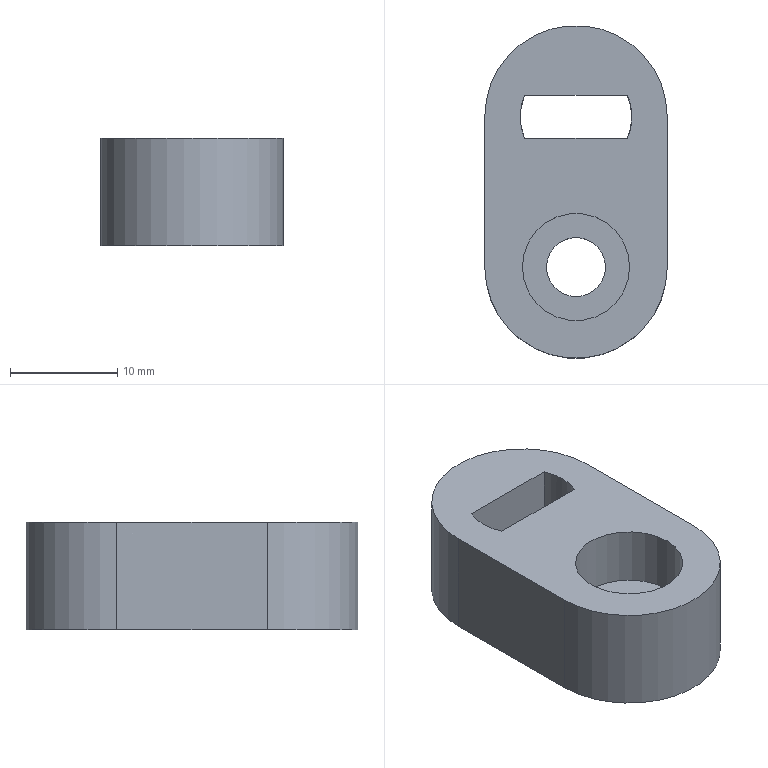Part | STEP file | lll_id290_x_t | 1 solid | 14 faces | box 17 x 31 x 10 mm | volume 3483 mm3 | plane 9 | cylinder 5 | commonest cylinder face diameters 17 x2 5.5 x1 10 x1 10.4 x1
STEP:
#1=CARTESIAN_POINT('',(5.,92.,-10.));
#2=VERTEX_POINT('',#1);
#3=CARTESIAN_POINT('',(0.,92.,-10.));
#4=DIRECTION('',(0.,0.,-1.));
#5=DIRECTION('',(1.,0.,0.));
#6=AXIS2_PLACEMENT_3D('',#3,#4,#5);
#7=CIRCLE('',#6,5.);
#8=EDGE_CURVE('',#2,#2,#7,.T.);
#9=ORIENTED_EDGE('',*,*,#8,.T.);
#10=EDGE_LOOP('',(#9));
#11=FACE_BOUND('',#10,.T.);
#12=CARTESIAN_POINT('',(-4.8,108.,-10.));
#13=VERTEX_POINT('',#12);
#14=CARTESIAN_POINT('',(-4.8,104.,-10.));
#15=VERTEX_POINT('',#14);
#16=CARTESIAN_POINT('',(0.,106.,-10.));
#17=DIRECTION('',(0.,0.,1.));
#18=DIRECTION('',(-1.,0.,0.));
#19=AXIS2_PLACEMENT_3D('',#16,#17,#18);
#20=CIRCLE('',#19,5.2);
#21=EDGE_CURVE('',#13,#15,#20,.T.);
#22=ORIENTED_EDGE('',*,*,#21,.F.);
#23=CARTESIAN_POINT('',(4.8,108.,-10.));
#24=VERTEX_POINT('',#23);
#25=CARTESIAN_POINT('',(0.,108.,-10.));
#26=DIRECTION('',(1.,0.,0.));
#27=VECTOR('',#26,1.);
#28=LINE('',#25,#27);
#29=EDGE_CURVE('',#13,#24,#28,.T.);
#30=ORIENTED_EDGE('',*,*,#29,.T.);
#31=CARTESIAN_POINT('',(4.8,104.,-10.));
#32=VERTEX_POINT('',#31);
#33=CARTESIAN_POINT('',(0.,106.,-10.));
#34=DIRECTION('',(0.,0.,1.));
#35=DIRECTION('',(-1.,0.,0.));
#36=AXIS2_PLACEMENT_3D('',#33,#34,#35);
#37=CIRCLE('',#36,5.2);
#38=EDGE_CURVE('',#32,#24,#37,.T.);
#39=ORIENTED_EDGE('',*,*,#38,.F.);
#40=CARTESIAN_POINT('',(0.,104.,-10.));
#41=DIRECTION('',(-1.,0.,0.));
#42=VECTOR('',#41,1.);
#43=LINE('',#40,#42);
#44=EDGE_CURVE('',#32,#15,#43,.T.);
#45=ORIENTED_EDGE('',*,*,#44,.T.);
#46=EDGE_LOOP('',(#22,#30,#39,#45));
#47=FACE_BOUND('',#46,.T.);
#48=CARTESIAN_POINT('',(-8.5,106.,-10.));
#49=VERTEX_POINT('',#48);
#50=CARTESIAN_POINT('',(8.5,106.,-10.));
#51=VERTEX_POINT('',#50);
#52=CARTESIAN_POINT('',(0.,106.,-10.));
#53=DIRECTION('',(0.,0.,-1.));
#54=DIRECTION('',(-1.,0.,0.));
#55=AXIS2_PLACEMENT_3D('',#52,#53,#54);
#56=CIRCLE('',#55,8.5);
#57=EDGE_CURVE('',#49,#51,#56,.T.);
#58=ORIENTED_EDGE('',*,*,#57,.F.);
#59=CARTESIAN_POINT('',(-8.5,92.,-10.));
#60=VERTEX_POINT('',#59);
#61=CARTESIAN_POINT('',(-8.5,94.,-10.));
#62=DIRECTION('',(0.,1.,0.));
#63=VECTOR('',#62,1.);
#64=LINE('',#61,#63);
#65=EDGE_CURVE('',#60,#49,#64,.T.);
#66=ORIENTED_EDGE('',*,*,#65,.F.);
#67=CARTESIAN_POINT('',(8.5,92.,-10.));
#68=VERTEX_POINT('',#67);
#69=CARTESIAN_POINT('',(0.,92.,-10.));
#70=DIRECTION('',(0.,0.,-1.));
#71=DIRECTION('',(-1.,0.,0.));
#72=AXIS2_PLACEMENT_3D('',#69,#70,#71);
#73=CIRCLE('',#72,8.5);
#74=EDGE_CURVE('',#68,#60,#73,.T.);
#75=ORIENTED_EDGE('',*,*,#74,.F.);
#76=CARTESIAN_POINT('',(8.5,94.,-10.));
#77=DIRECTION('',(0.,-1.,0.));
#78=VECTOR('',#77,1.);
#79=LINE('',#76,#78);
#80=EDGE_CURVE('',#51,#68,#79,.T.);
#81=ORIENTED_EDGE('',*,*,#80,.F.);
#82=EDGE_LOOP('',(#58,#66,#75,#81));
#83=FACE_BOUND('',#82,.T.);
#84=CARTESIAN_POINT('',(0.,94.,-10.));
#85=DIRECTION('',(0.,0.,1.));
#86=DIRECTION('',(0.,1.,0.));
#87=AXIS2_PLACEMENT_3D('',#84,#85,#86);
#88=PLANE('',#87);
#89=ADVANCED_FACE('',(#11,#47,#83),#88,.T.);
#90=CARTESIAN_POINT('',(8.5,92.,-20.));
#91=VERTEX_POINT('',#90);
#92=CARTESIAN_POINT('',(8.5,92.,-20.));
#93=DIRECTION('',(0.,0.,-1.));
#94=VECTOR('',#93,1.);
#95=LINE('',#92,#94);
#96=EDGE_CURVE('',#68,#91,#95,.T.);
#97=ORIENTED_EDGE('',*,*,#96,.T.);
#98=CARTESIAN_POINT('',(8.5,106.,-20.));
#99=VERTEX_POINT('',#98);
#100=CARTESIAN_POINT('',(8.5,94.,-20.));
#101=DIRECTION('',(0.,1.,0.));
#102=VECTOR('',#101,1.);
#103=LINE('',#100,#102);
#104=EDGE_CURVE('',#91,#99,#103,.T.);
#105=ORIENTED_EDGE('',*,*,#104,.T.);
#106=CARTESIAN_POINT('',(8.5,106.,-20.));
#107=DIRECTION('',(0.,0.,1.));
#108=VECTOR('',#107,1.);
#109=LINE('',#106,#108);
#110=EDGE_CURVE('',#99,#51,#109,.T.);
#111=ORIENTED_EDGE('',*,*,#110,.T.);
#112=ORIENTED_EDGE('',*,*,#80,.T.);
#113=EDGE_LOOP('',(#97,#105,#111,#112));
#114=FACE_OUTER_BOUND('',#113,.T.);
#115=CARTESIAN_POINT('',(8.5,94.,-20.));
#116=DIRECTION('',(1.,0.,0.));
#117=DIRECTION('',(0.,0.,-1.));
#118=AXIS2_PLACEMENT_3D('',#115,#116,#117);
#119=PLANE('',#118);
#120=ADVANCED_FACE('',(#114),#119,.T.);
#121=CARTESIAN_POINT('',(-8.5,106.,-20.));
#122=VERTEX_POINT('',#121);
#123=CARTESIAN_POINT('',(-8.5,106.,-20.));
#124=DIRECTION('',(0.,0.,-1.));
#125=VECTOR('',#124,1.);
#126=LINE('',#123,#125);
#127=EDGE_CURVE('',#49,#122,#126,.T.);
#128=ORIENTED_EDGE('',*,*,#127,.T.);
#129=CARTESIAN_POINT('',(-8.5,92.,-20.));
#130=VERTEX_POINT('',#129);
#131=CARTESIAN_POINT('',(-8.5,94.,-20.));
#132=DIRECTION('',(0.,-1.,0.));
#133=VECTOR('',#132,1.);
#134=LINE('',#131,#133);
#135=EDGE_CURVE('',#122,#130,#134,.T.);
#136=ORIENTED_EDGE('',*,*,#135,.T.);
#137=CARTESIAN_POINT('',(-8.5,92.,-20.));
#138=DIRECTION('',(0.,0.,1.));
#139=VECTOR('',#138,1.);
#140=LINE('',#137,#139);
#141=EDGE_CURVE('',#130,#60,#140,.T.);
#142=ORIENTED_EDGE('',*,*,#141,.T.);
#143=ORIENTED_EDGE('',*,*,#65,.T.);
#144=EDGE_LOOP('',(#128,#136,#142,#143));
#145=FACE_OUTER_BOUND('',#144,.T.);
#146=CARTESIAN_POINT('',(-8.5,94.,-20.));
#147=DIRECTION('',(-1.,0.,0.));
#148=DIRECTION('',(0.,0.,1.));
#149=AXIS2_PLACEMENT_3D('',#146,#147,#148);
#150=PLANE('',#149);
#151=ADVANCED_FACE('',(#145),#150,.T.);
#152=CARTESIAN_POINT('',(2.75,92.,-20.));
#153=VERTEX_POINT('',#152);
#154=CARTESIAN_POINT('',(0.,92.,-20.));
#155=DIRECTION('',(0.,0.,-1.));
#156=DIRECTION('',(1.,0.,0.));
#157=AXIS2_PLACEMENT_3D('',#154,#155,#156);
#158=CIRCLE('',#157,2.75);
#159=EDGE_CURVE('',#153,#153,#158,.T.);
#160=ORIENTED_EDGE('',*,*,#159,.F.);
#161=EDGE_LOOP('',(#160));
#162=FACE_BOUND('',#161,.T.);
#163=CARTESIAN_POINT('',(5.2,106.,-20.));
#164=VERTEX_POINT('',#163);
#165=CARTESIAN_POINT('',(0.,106.,-20.));
#166=DIRECTION('',(0.,0.,1.));
#167=DIRECTION('',(1.,0.,0.));
#168=AXIS2_PLACEMENT_3D('',#165,#166,#167);
#169=CIRCLE('',#168,5.2);
#170=EDGE_CURVE('',#164,#164,#169,.T.);
#171=ORIENTED_EDGE('',*,*,#170,.T.);
#172=EDGE_LOOP('',(#171));
#173=FACE_BOUND('',#172,.T.);
#174=ORIENTED_EDGE('',*,*,#135,.F.);
#175=CARTESIAN_POINT('',(0.,106.,-20.));
#176=DIRECTION('',(0.,0.,1.));
#177=DIRECTION('',(1.,0.,0.));
#178=AXIS2_PLACEMENT_3D('',#175,#176,#177);
#179=CIRCLE('',#178,8.5);
#180=EDGE_CURVE('',#99,#122,#179,.T.);
#181=ORIENTED_EDGE('',*,*,#180,.F.);
#182=ORIENTED_EDGE('',*,*,#104,.F.);
#183=CARTESIAN_POINT('',(0.,92.,-20.));
#184=DIRECTION('',(0.,0.,1.));
#185=DIRECTION('',(1.,0.,0.));
#186=AXIS2_PLACEMENT_3D('',#183,#184,#185);
#187=CIRCLE('',#186,8.5);
#188=EDGE_CURVE('',#130,#91,#187,.T.);
#189=ORIENTED_EDGE('',*,*,#188,.F.);
#190=EDGE_LOOP('',(#174,#181,#182,#189));
#191=FACE_BOUND('',#190,.T.);
#192=CARTESIAN_POINT('',(0.,94.,-20.));
#193=DIRECTION('',(0.,0.,-1.));
#194=DIRECTION('',(0.,-1.,0.));
#195=AXIS2_PLACEMENT_3D('',#192,#193,#194);
#196=PLANE('',#195);
#197=ADVANCED_FACE('',(#162,#173,#191),#196,.T.);
#198=ORIENTED_EDGE('',*,*,#141,.F.);
#199=ORIENTED_EDGE('',*,*,#188,.T.);
#200=ORIENTED_EDGE('',*,*,#96,.F.);
#201=ORIENTED_EDGE('',*,*,#74,.T.);
#202=EDGE_LOOP('',(#198,#199,#200,#201));
#203=FACE_OUTER_BOUND('',#202,.T.);
#204=CARTESIAN_POINT('',(0.,92.,-20.));
#205=DIRECTION('',(0.,0.,1.));
#206=DIRECTION('',(0.,1.,0.));
#207=AXIS2_PLACEMENT_3D('',#204,#205,#206);
#208=CYLINDRICAL_SURFACE('',#207,8.5);
#209=ADVANCED_FACE('',(#203),#208,.T.);
#210=ORIENTED_EDGE('',*,*,#110,.F.);
#211=ORIENTED_EDGE('',*,*,#180,.T.);
#212=ORIENTED_EDGE('',*,*,#127,.F.);
#213=ORIENTED_EDGE('',*,*,#57,.T.);
#214=EDGE_LOOP('',(#210,#211,#212,#213));
#215=FACE_OUTER_BOUND('',#214,.T.);
#216=CARTESIAN_POINT('',(0.,106.,-20.));
#217=DIRECTION('',(0.,0.,1.));
#218=DIRECTION('',(0.,-1.,0.));
#219=AXIS2_PLACEMENT_3D('',#216,#217,#218);
#220=CYLINDRICAL_SURFACE('',#219,8.5);
#221=ADVANCED_FACE('',(#215),#220,.T.);
#222=CARTESIAN_POINT('',(4.8,104.,-15.));
#223=VERTEX_POINT('',#222);
#224=CARTESIAN_POINT('',(4.8,104.,-20.));
#225=DIRECTION('',(0.,0.,-1.));
#226=VECTOR('',#225,1.);
#227=LINE('',#224,#226);
#228=EDGE_CURVE('',#32,#223,#227,.T.);
#229=ORIENTED_EDGE('',*,*,#228,.T.);
#230=CARTESIAN_POINT('',(-4.8,104.,-15.));
#231=VERTEX_POINT('',#230);
#232=CARTESIAN_POINT('',(13.,104.,-15.));
#233=DIRECTION('',(-1.,0.,0.));
#234=VECTOR('',#233,1.);
#235=LINE('',#232,#234);
#236=EDGE_CURVE('',#223,#231,#235,.T.);
#237=ORIENTED_EDGE('',*,*,#236,.T.);
#238=CARTESIAN_POINT('',(-4.8,104.,-15.));
#239=DIRECTION('',(0.,0.,1.));
#240=VECTOR('',#239,1.);
#241=LINE('',#238,#240);
#242=EDGE_CURVE('',#231,#15,#241,.T.);
#243=ORIENTED_EDGE('',*,*,#242,.T.);
#244=ORIENTED_EDGE('',*,*,#44,.F.);
#245=EDGE_LOOP('',(#229,#237,#243,#244));
#246=FACE_OUTER_BOUND('',#245,.T.);
#247=CARTESIAN_POINT('',(13.,104.,-9.5));
#248=DIRECTION('',(0.,1.,0.));
#249=DIRECTION('',(0.,0.,-1.));
#250=AXIS2_PLACEMENT_3D('',#247,#248,#249);
#251=PLANE('',#250);
#252=ADVANCED_FACE('',(#246),#251,.T.);
#253=CARTESIAN_POINT('',(-4.8,108.,-15.));
#254=VERTEX_POINT('',#253);
#255=CARTESIAN_POINT('',(4.8,108.,-15.));
#256=VERTEX_POINT('',#255);
#257=CARTESIAN_POINT('',(0.,106.,-15.));
#258=DIRECTION('',(0.,0.,-1.));
#259=DIRECTION('',(1.,0.,0.));
#260=AXIS2_PLACEMENT_3D('',#257,#258,#259);
#261=CIRCLE('',#260,5.2);
#262=EDGE_CURVE('',#254,#256,#261,.T.);
#263=ORIENTED_EDGE('',*,*,#262,.T.);
#264=CARTESIAN_POINT('',(13.,108.,-15.));
#265=DIRECTION('',(-1.,0.,0.));
#266=VECTOR('',#265,1.);
#267=LINE('',#264,#266);
#268=EDGE_CURVE('',#256,#254,#267,.T.);
#269=ORIENTED_EDGE('',*,*,#268,.T.);
#270=EDGE_LOOP('',(#263,#269));
#271=FACE_OUTER_BOUND('',#270,.T.);
#272=CARTESIAN_POINT('',(13.,111.,-15.));
#273=DIRECTION('',(0.,0.,-1.));
#274=DIRECTION('',(0.,-1.,0.));
#275=AXIS2_PLACEMENT_3D('',#272,#273,#274);
#276=PLANE('',#275);
#277=ADVANCED_FACE('',(#271),#276,.T.);
#278=CARTESIAN_POINT('',(-4.8,108.,-20.));
#279=DIRECTION('',(0.,0.,-1.));
#280=VECTOR('',#279,1.);
#281=LINE('',#278,#280);
#282=EDGE_CURVE('',#13,#254,#281,.T.);
#283=ORIENTED_EDGE('',*,*,#282,.T.);
#284=ORIENTED_EDGE('',*,*,#268,.F.);
#285=CARTESIAN_POINT('',(4.8,108.,-20.));
#286=DIRECTION('',(0.,0.,1.));
#287=VECTOR('',#286,1.);
#288=LINE('',#285,#287);
#289=EDGE_CURVE('',#256,#24,#288,.T.);
#290=ORIENTED_EDGE('',*,*,#289,.T.);
#291=ORIENTED_EDGE('',*,*,#29,.F.);
#292=EDGE_LOOP('',(#283,#284,#290,#291));
#293=FACE_OUTER_BOUND('',#292,.T.);
#294=CARTESIAN_POINT('',(13.,108.,-15.));
#295=DIRECTION('',(0.,-1.,0.));
#296=DIRECTION('',(0.,0.,1.));
#297=AXIS2_PLACEMENT_3D('',#294,#295,#296);
#298=PLANE('',#297);
#299=ADVANCED_FACE('',(#293),#298,.T.);
#300=CARTESIAN_POINT('',(0.,106.,-15.));
#301=DIRECTION('',(0.,0.,-1.));
#302=DIRECTION('',(1.,0.,0.));
#303=AXIS2_PLACEMENT_3D('',#300,#301,#302);
#304=CIRCLE('',#303,5.2);
#305=EDGE_CURVE('',#223,#231,#304,.T.);
#306=ORIENTED_EDGE('',*,*,#305,.T.);
#307=ORIENTED_EDGE('',*,*,#236,.F.);
#308=EDGE_LOOP('',(#306,#307));
#309=FACE_OUTER_BOUND('',#308,.T.);
#310=CARTESIAN_POINT('',(13.,104.,-15.));
#311=DIRECTION('',(0.,0.,-1.));
#312=DIRECTION('',(0.,-1.,0.));
#313=AXIS2_PLACEMENT_3D('',#310,#311,#312);
#314=PLANE('',#313);
#315=ADVANCED_FACE('',(#309),#314,.T.);
#316=ORIENTED_EDGE('',*,*,#21,.T.);
#317=ORIENTED_EDGE('',*,*,#242,.F.);
#318=ORIENTED_EDGE('',*,*,#305,.F.);
#319=ORIENTED_EDGE('',*,*,#228,.F.);
#320=ORIENTED_EDGE('',*,*,#38,.T.);
#321=ORIENTED_EDGE('',*,*,#289,.F.);
#322=ORIENTED_EDGE('',*,*,#262,.F.);
#323=ORIENTED_EDGE('',*,*,#282,.F.);
#324=EDGE_LOOP('',(#316,#317,#318,#319,#320,#321,#322,#323));
#325=FACE_BOUND('',#324,.T.);
#326=ORIENTED_EDGE('',*,*,#170,.F.);
#327=EDGE_LOOP('',(#326));
#328=FACE_BOUND('',#327,.T.);
#329=CARTESIAN_POINT('',(0.,106.,-20.));
#330=DIRECTION('',(0.,0.,1.));
#331=DIRECTION('',(1.,0.,0.));
#332=AXIS2_PLACEMENT_3D('',#329,#330,#331);
#333=CYLINDRICAL_SURFACE('',#332,5.2);
#334=ADVANCED_FACE('',(#325,#328),#333,.F.);
#335=ORIENTED_EDGE('',*,*,#159,.T.);
#336=EDGE_LOOP('',(#335));
#337=FACE_BOUND('',#336,.T.);
#338=CARTESIAN_POINT('',(2.75,92.,-15.5));
#339=VERTEX_POINT('',#338);
#340=CARTESIAN_POINT('',(0.,92.,-15.5));
#341=DIRECTION('',(0.,0.,-1.));
#342=DIRECTION('',(1.,0.,0.));
#343=AXIS2_PLACEMENT_3D('',#340,#341,#342);
#344=CIRCLE('',#343,2.75);
#345=EDGE_CURVE('',#339,#339,#344,.T.);
#346=ORIENTED_EDGE('',*,*,#345,.F.);
#347=EDGE_LOOP('',(#346));
#348=FACE_BOUND('',#347,.T.);
#349=CARTESIAN_POINT('',(0.,92.,-310.));
#350=DIRECTION('',(0.,0.,-1.));
#351=DIRECTION('',(1.,0.,0.));
#352=AXIS2_PLACEMENT_3D('',#349,#350,#351);
#353=CYLINDRICAL_SURFACE('',#352,2.75);
#354=ADVANCED_FACE('',(#337,#348),#353,.F.);
#355=ORIENTED_EDGE('',*,*,#345,.T.);
#356=EDGE_LOOP('',(#355));
#357=FACE_BOUND('',#356,.T.);
#358=CARTESIAN_POINT('',(5.,92.,-15.5));
#359=VERTEX_POINT('',#358);
#360=CARTESIAN_POINT('',(0.,92.,-15.5));
#361=DIRECTION('',(0.,0.,-1.));
#362=DIRECTION('',(1.,0.,0.));
#363=AXIS2_PLACEMENT_3D('',#360,#361,#362);
#364=CIRCLE('',#363,5.);
#365=EDGE_CURVE('',#359,#359,#364,.T.);
#366=ORIENTED_EDGE('',*,*,#365,.F.);
#367=EDGE_LOOP('',(#366));
#368=FACE_BOUND('',#367,.T.);
#369=CARTESIAN_POINT('',(0.,95.,-15.5));
#370=DIRECTION('',(0.,0.,-1.));
#371=DIRECTION('',(1.,0.,0.));
#372=AXIS2_PLACEMENT_3D('',#369,#370,#371);
#373=PLANE('',#372);
#374=ADVANCED_FACE('',(#357,#368),#373,.F.);
#375=ORIENTED_EDGE('',*,*,#365,.T.);
#376=EDGE_LOOP('',(#375));
#377=FACE_BOUND('',#376,.T.);
#378=ORIENTED_EDGE('',*,*,#8,.F.);
#379=EDGE_LOOP('',(#378));
#380=FACE_BOUND('',#379,.T.);
#381=CARTESIAN_POINT('',(0.,92.,-10.));
#382=DIRECTION('',(0.,0.,-1.));
#383=DIRECTION('',(1.,0.,0.));
#384=AXIS2_PLACEMENT_3D('',#381,#382,#383);
#385=CYLINDRICAL_SURFACE('',#384,5.);
#386=ADVANCED_FACE('',(#377,#380),#385,.F.);
#387=CLOSED_SHELL('',(#89,#120,#151,#197,#209,#221,#252,#277,#299,#315,#334,#354,#374,#386));
#388=MANIFOLD_SOLID_BREP('',#387);
#389=(LENGTH_UNIT()NAMED_UNIT(*)SI_UNIT(.MILLI.,.METRE.));
#390=UNCERTAINTY_MEASURE_WITH_UNIT(LENGTH_MEASURE(0.00002),#389,'','');
#391=(NAMED_UNIT(*)PLANE_ANGLE_UNIT()SI_UNIT($,.RADIAN.));
#392=PLANE_ANGLE_MEASURE_WITH_UNIT(PLANE_ANGLE_MEASURE(0.01745),#391);
#393=DIMENSIONAL_EXPONENTS(0.,0.,0.,0.,0.,0.,0.);
#394=(CONVERSION_BASED_UNIT('DEGREE',#392)NAMED_UNIT(#393)PLANE_ANGLE_UNIT());
#395=(NAMED_UNIT(*)SI_UNIT($,.STERADIAN.)SOLID_ANGLE_UNIT());
#396=(GEOMETRIC_REPRESENTATION_CONTEXT(3)GLOBAL_UNCERTAINTY_ASSIGNED_CONTEXT((#390))GLOBAL_UNIT_ASSIGNED_CONTEXT((#389,#394,#395))REPRESENTATION_CONTEXT('',''));
#397=ADVANCED_BREP_SHAPE_REPRESENTATION('',(#388),#396);